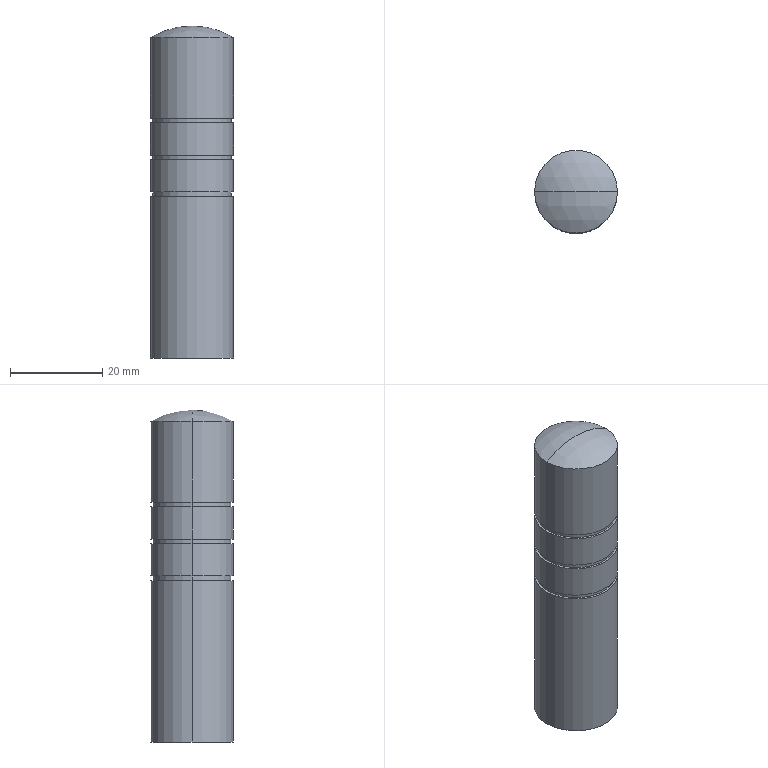Part | SolidWorks | features ICE 4, Extrusion 1, HoleWzd 1, Revolution 1 | 1 solid | 32 faces | box 18 x 18 x 71.992 mm | volume 12874 mm3 | cylinder 18 | plane 8 | cone 4 | sphere 2 | commonest cylinder face diameters 18 x8 17 x6 4.2 x2 14 x2
STEP:
#1=CARTESIAN_POINT('',(2.1,0.,32.425));
#2=VERTEX_POINT('',#1);
#3=CARTESIAN_POINT('',(-2.1,0.,32.425));
#4=VERTEX_POINT('',#3);
#5=CARTESIAN_POINT('',(0.,0.,32.425));
#6=DIRECTION('',(0.,0.,-1.));
#7=DIRECTION('',(-1.,0.,0.));
#8=AXIS2_PLACEMENT_3D('',#5,#6,#7);
#9=CIRCLE('',#8,2.1);
#10=EDGE_CURVE('',#2,#4,#9,.T.);
#11=ORIENTED_EDGE('',*,*,#10,.F.);
#12=CARTESIAN_POINT('',(2.525,0.,32.));
#13=VERTEX_POINT('',#12);
#14=CARTESIAN_POINT('',(2.525,0.,32.));
#15=DIRECTION('',(0.7071,0.,-0.7071));
#16=VECTOR('',#15,1000.);
#17=LINE('',#14,#16);
#18=EDGE_CURVE('',#2,#13,#17,.T.);
#19=ORIENTED_EDGE('',*,*,#18,.T.);
#20=CARTESIAN_POINT('',(-2.525,0.,32.));
#21=VERTEX_POINT('',#20);
#22=CARTESIAN_POINT('',(0.,0.,32.));
#23=DIRECTION('',(0.,0.,-1.));
#24=DIRECTION('',(-1.,0.,0.));
#25=AXIS2_PLACEMENT_3D('',#22,#23,#24);
#26=CIRCLE('',#25,2.525);
#27=EDGE_CURVE('',#13,#21,#26,.T.);
#28=ORIENTED_EDGE('',*,*,#27,.T.);
#29=CARTESIAN_POINT('',(-2.525,0.,32.));
#30=DIRECTION('',(-0.7071,0.,-0.7071));
#31=VECTOR('',#30,1000.);
#32=LINE('',#29,#31);
#33=EDGE_CURVE('',#4,#21,#32,.T.);
#34=ORIENTED_EDGE('',*,*,#33,.F.);
#35=EDGE_LOOP('',(#11,#19,#28,#34));
#36=FACE_OUTER_BOUND('',#35,.T.);
#37=CARTESIAN_POINT('',(0.,0.,32.));
#38=DIRECTION('',(0.,0.,-1.));
#39=DIRECTION('',(-1.,0.,0.));
#40=AXIS2_PLACEMENT_3D('',#37,#38,#39);
#41=CONICAL_SURFACE('',#40,2.525,0.7854);
#42=ADVANCED_FACE('',(#36),#41,.F.);
#43=CARTESIAN_POINT('',(2.1,0.,40.738));
#44=VERTEX_POINT('',#43);
#45=CARTESIAN_POINT('',(-2.1,0.,40.738));
#46=VERTEX_POINT('',#45);
#47=CARTESIAN_POINT('',(0.,0.,40.738));
#48=DIRECTION('',(0.,0.,-1.));
#49=DIRECTION('',(-1.,0.,0.));
#50=AXIS2_PLACEMENT_3D('',#47,#48,#49);
#51=CIRCLE('',#50,2.1);
#52=EDGE_CURVE('',#44,#46,#51,.T.);
#53=ORIENTED_EDGE('',*,*,#52,.F.);
#54=CARTESIAN_POINT('',(2.1,0.,32.));
#55=DIRECTION('',(0.,0.,-1.));
#56=VECTOR('',#55,1000.);
#57=LINE('',#54,#56);
#58=EDGE_CURVE('',#44,#2,#57,.T.);
#59=ORIENTED_EDGE('',*,*,#58,.T.);
#60=ORIENTED_EDGE('',*,*,#10,.T.);
#61=CARTESIAN_POINT('',(-2.1,0.,32.));
#62=DIRECTION('',(0.,0.,-1.));
#63=VECTOR('',#62,1000.);
#64=LINE('',#61,#63);
#65=EDGE_CURVE('',#46,#4,#64,.T.);
#66=ORIENTED_EDGE('',*,*,#65,.F.);
#67=EDGE_LOOP('',(#53,#59,#60,#66));
#68=FACE_OUTER_BOUND('',#67,.T.);
#69=CARTESIAN_POINT('',(0.,0.,32.));
#70=DIRECTION('',(0.,0.,-1.));
#71=DIRECTION('',(-1.,0.,0.));
#72=AXIS2_PLACEMENT_3D('',#69,#70,#71);
#73=CYLINDRICAL_SURFACE('',#72,2.1);
#74=ADVANCED_FACE('',(#68),#73,.F.);
#75=CARTESIAN_POINT('',(0.,0.,42.));
#76=VERTEX_POINT('',#75);
#77=CARTESIAN_POINT('',(-2.1,0.,40.738));
#78=DIRECTION('',(-0.8572,0.,-0.515));
#79=VECTOR('',#78,1000.);
#80=LINE('',#77,#79);
#81=EDGE_CURVE('',#76,#46,#80,.T.);
#82=ORIENTED_EDGE('',*,*,#81,.F.);
#83=CARTESIAN_POINT('',(2.1,0.,40.738));
#84=DIRECTION('',(0.8572,0.,-0.515));
#85=VECTOR('',#84,1000.);
#86=LINE('',#83,#85);
#87=EDGE_CURVE('',#76,#44,#86,.T.);
#88=ORIENTED_EDGE('',*,*,#87,.T.);
#89=ORIENTED_EDGE('',*,*,#52,.T.);
#90=EDGE_LOOP('',(#82,#88,#89));
#91=FACE_OUTER_BOUND('',#90,.T.);
#92=CARTESIAN_POINT('',(0.,0.,40.738));
#93=DIRECTION('',(0.,0.,-1.));
#94=DIRECTION('',(-1.,0.,0.));
#95=AXIS2_PLACEMENT_3D('',#92,#93,#94);
#96=CONICAL_SURFACE('',#95,2.1,1.03);
#97=ADVANCED_FACE('',(#91),#96,.F.);
#98=CARTESIAN_POINT('',(0.,0.,71.992));
#99=VERTEX_POINT('',#98);
#100=CARTESIAN_POINT('',(-9.,0.,69.5));
#101=VERTEX_POINT('',#100);
#102=CARTESIAN_POINT('',(0.,0.,54.492));
#103=DIRECTION('',(0.,-1.,0.));
#104=DIRECTION('',(0.,0.,-1.));
#105=AXIS2_PLACEMENT_3D('',#102,#103,#104);
#106=CIRCLE('',#105,17.5);
#107=EDGE_CURVE('',#99,#101,#106,.T.);
#108=ORIENTED_EDGE('',*,*,#107,.F.);
#109=CARTESIAN_POINT('',(9.,0.,69.5));
#110=VERTEX_POINT('',#109);
#111=CARTESIAN_POINT('',(0.,0.,54.492));
#112=DIRECTION('',(0.,1.,0.));
#113=DIRECTION('',(-1.,0.,0.));
#114=AXIS2_PLACEMENT_3D('',#111,#112,#113);
#115=CIRCLE('',#114,17.5);
#116=EDGE_CURVE('',#99,#110,#115,.T.);
#117=ORIENTED_EDGE('',*,*,#116,.T.);
#118=CARTESIAN_POINT('',(0.,0.,69.5));
#119=DIRECTION('',(0.,0.,1.));
#120=DIRECTION('',(1.,0.,0.));
#121=AXIS2_PLACEMENT_3D('',#118,#119,#120);
#122=CIRCLE('',#121,9.);
#123=EDGE_CURVE('',#110,#101,#122,.T.);
#124=ORIENTED_EDGE('',*,*,#123,.T.);
#125=EDGE_LOOP('',(#108,#117,#124));
#126=FACE_OUTER_BOUND('',#125,.T.);
#127=CARTESIAN_POINT('',(0.,0.,54.492));
#128=DIRECTION('',(0.,1.,0.));
#129=DIRECTION('',(-1.,0.,0.));
#130=AXIS2_PLACEMENT_3D('',#127,#128,#129);
#131=SPHERICAL_SURFACE('',#130,17.5);
#132=ADVANCED_FACE('',(#126),#131,.T.);
#133=ORIENTED_EDGE('',*,*,#123,.F.);
#134=CARTESIAN_POINT('',(9.,0.,52.));
#135=VERTEX_POINT('',#134);
#136=CARTESIAN_POINT('',(9.,0.,69.5));
#137=DIRECTION('',(0.,0.,-1.));
#138=VECTOR('',#137,1000.);
#139=LINE('',#136,#138);
#140=EDGE_CURVE('',#110,#135,#139,.T.);
#141=ORIENTED_EDGE('',*,*,#140,.T.);
#142=CARTESIAN_POINT('',(-9.,0.,52.));
#143=VERTEX_POINT('',#142);
#144=CARTESIAN_POINT('',(0.,0.,52.));
#145=DIRECTION('',(0.,0.,-1.));
#146=DIRECTION('',(-1.,0.,0.));
#147=AXIS2_PLACEMENT_3D('',#144,#145,#146);
#148=CIRCLE('',#147,9.);
#149=EDGE_CURVE('',#143,#135,#148,.T.);
#150=ORIENTED_EDGE('',*,*,#149,.F.);
#151=CARTESIAN_POINT('',(-9.,0.,69.5));
#152=DIRECTION('',(0.,0.,-1.));
#153=VECTOR('',#152,1000.);
#154=LINE('',#151,#153);
#155=EDGE_CURVE('',#101,#143,#154,.T.);
#156=ORIENTED_EDGE('',*,*,#155,.F.);
#157=EDGE_LOOP('',(#133,#141,#150,#156));
#158=FACE_OUTER_BOUND('',#157,.T.);
#159=CARTESIAN_POINT('',(0.,0.,69.5));
#160=DIRECTION('',(0.,0.,-1.));
#161=DIRECTION('',(-1.,0.,0.));
#162=AXIS2_PLACEMENT_3D('',#159,#160,#161);
#163=CYLINDRICAL_SURFACE('',#162,9.);
#164=ADVANCED_FACE('',(#158),#163,.T.);
#165=CARTESIAN_POINT('',(-8.5,0.,52.));
#166=VERTEX_POINT('',#165);
#167=CARTESIAN_POINT('',(8.5,0.,52.));
#168=VERTEX_POINT('',#167);
#169=CARTESIAN_POINT('',(0.,0.,52.));
#170=DIRECTION('',(0.,0.,-1.));
#171=DIRECTION('',(-1.,0.,0.));
#172=AXIS2_PLACEMENT_3D('',#169,#170,#171);
#173=CIRCLE('',#172,8.5);
#174=EDGE_CURVE('',#166,#168,#173,.T.);
#175=ORIENTED_EDGE('',*,*,#174,.T.);
#176=CARTESIAN_POINT('',(8.5,0.,51.));
#177=VERTEX_POINT('',#176);
#178=CARTESIAN_POINT('',(8.5,0.,52.));
#179=DIRECTION('',(0.,0.,-1.));
#180=VECTOR('',#179,1000.);
#181=LINE('',#178,#180);
#182=EDGE_CURVE('',#168,#177,#181,.T.);
#183=ORIENTED_EDGE('',*,*,#182,.T.);
#184=CARTESIAN_POINT('',(-8.5,0.,51.));
#185=VERTEX_POINT('',#184);
#186=CARTESIAN_POINT('',(0.,0.,51.));
#187=DIRECTION('',(0.,0.,-1.));
#188=DIRECTION('',(-1.,0.,0.));
#189=AXIS2_PLACEMENT_3D('',#186,#187,#188);
#190=CIRCLE('',#189,8.5);
#191=EDGE_CURVE('',#185,#177,#190,.T.);
#192=ORIENTED_EDGE('',*,*,#191,.F.);
#193=CARTESIAN_POINT('',(-8.5,0.,52.));
#194=DIRECTION('',(0.,0.,-1.));
#195=VECTOR('',#194,1000.);
#196=LINE('',#193,#195);
#197=EDGE_CURVE('',#166,#185,#196,.T.);
#198=ORIENTED_EDGE('',*,*,#197,.F.);
#199=EDGE_LOOP('',(#175,#183,#192,#198));
#200=FACE_OUTER_BOUND('',#199,.T.);
#201=CARTESIAN_POINT('',(0.,0.,52.));
#202=DIRECTION('',(0.,0.,-1.));
#203=DIRECTION('',(-1.,0.,0.));
#204=AXIS2_PLACEMENT_3D('',#201,#202,#203);
#205=CYLINDRICAL_SURFACE('',#204,8.5);
#206=ADVANCED_FACE('',(#200),#205,.T.);
#207=CARTESIAN_POINT('',(-9.,0.,51.));
#208=VERTEX_POINT('',#207);
#209=CARTESIAN_POINT('',(9.,0.,51.));
#210=VERTEX_POINT('',#209);
#211=CARTESIAN_POINT('',(0.,0.,51.));
#212=DIRECTION('',(0.,0.,-1.));
#213=DIRECTION('',(-1.,0.,0.));
#214=AXIS2_PLACEMENT_3D('',#211,#212,#213);
#215=CIRCLE('',#214,9.);
#216=EDGE_CURVE('',#208,#210,#215,.T.);
#217=ORIENTED_EDGE('',*,*,#216,.T.);
#218=CARTESIAN_POINT('',(9.,0.,44.));
#219=VERTEX_POINT('',#218);
#220=CARTESIAN_POINT('',(9.,0.,69.5));
#221=DIRECTION('',(0.,0.,-1.));
#222=VECTOR('',#221,1000.);
#223=LINE('',#220,#222);
#224=EDGE_CURVE('',#210,#219,#223,.T.);
#225=ORIENTED_EDGE('',*,*,#224,.T.);
#226=CARTESIAN_POINT('',(-9.,0.,44.));
#227=VERTEX_POINT('',#226);
#228=CARTESIAN_POINT('',(0.,0.,44.));
#229=DIRECTION('',(0.,0.,-1.));
#230=DIRECTION('',(-1.,0.,0.));
#231=AXIS2_PLACEMENT_3D('',#228,#229,#230);
#232=CIRCLE('',#231,9.);
#233=EDGE_CURVE('',#227,#219,#232,.T.);
#234=ORIENTED_EDGE('',*,*,#233,.F.);
#235=CARTESIAN_POINT('',(-9.,0.,69.5));
#236=DIRECTION('',(0.,0.,-1.));
#237=VECTOR('',#236,1000.);
#238=LINE('',#235,#237);
#239=EDGE_CURVE('',#208,#227,#238,.T.);
#240=ORIENTED_EDGE('',*,*,#239,.F.);
#241=EDGE_LOOP('',(#217,#225,#234,#240));
#242=FACE_OUTER_BOUND('',#241,.T.);
#243=CARTESIAN_POINT('',(0.,0.,69.5));
#244=DIRECTION('',(0.,0.,-1.));
#245=DIRECTION('',(-1.,0.,0.));
#246=AXIS2_PLACEMENT_3D('',#243,#244,#245);
#247=CYLINDRICAL_SURFACE('',#246,9.);
#248=ADVANCED_FACE('',(#242),#247,.T.);
#249=CARTESIAN_POINT('',(-8.5,0.,44.));
#250=VERTEX_POINT('',#249);
#251=CARTESIAN_POINT('',(8.5,0.,44.));
#252=VERTEX_POINT('',#251);
#253=CARTESIAN_POINT('',(0.,0.,44.));
#254=DIRECTION('',(0.,0.,-1.));
#255=DIRECTION('',(-1.,0.,0.));
#256=AXIS2_PLACEMENT_3D('',#253,#254,#255);
#257=CIRCLE('',#256,8.5);
#258=EDGE_CURVE('',#250,#252,#257,.T.);
#259=ORIENTED_EDGE('',*,*,#258,.T.);
#260=CARTESIAN_POINT('',(8.5,0.,43.));
#261=VERTEX_POINT('',#260);
#262=CARTESIAN_POINT('',(8.5,0.,44.));
#263=DIRECTION('',(0.,0.,-1.));
#264=VECTOR('',#263,1000.);
#265=LINE('',#262,#264);
#266=EDGE_CURVE('',#252,#261,#265,.T.);
#267=ORIENTED_EDGE('',*,*,#266,.T.);
#268=CARTESIAN_POINT('',(-8.5,0.,43.));
#269=VERTEX_POINT('',#268);
#270=CARTESIAN_POINT('',(0.,0.,43.));
#271=DIRECTION('',(0.,0.,-1.));
#272=DIRECTION('',(-1.,0.,0.));
#273=AXIS2_PLACEMENT_3D('',#270,#271,#272);
#274=CIRCLE('',#273,8.5);
#275=EDGE_CURVE('',#269,#261,#274,.T.);
#276=ORIENTED_EDGE('',*,*,#275,.F.);
#277=CARTESIAN_POINT('',(-8.5,0.,44.));
#278=DIRECTION('',(0.,0.,-1.));
#279=VECTOR('',#278,1000.);
#280=LINE('',#277,#279);
#281=EDGE_CURVE('',#250,#269,#280,.T.);
#282=ORIENTED_EDGE('',*,*,#281,.F.);
#283=EDGE_LOOP('',(#259,#267,#276,#282));
#284=FACE_OUTER_BOUND('',#283,.T.);
#285=CARTESIAN_POINT('',(0.,0.,44.));
#286=DIRECTION('',(0.,0.,-1.));
#287=DIRECTION('',(-1.,0.,0.));
#288=AXIS2_PLACEMENT_3D('',#285,#286,#287);
#289=CYLINDRICAL_SURFACE('',#288,8.5);
#290=ADVANCED_FACE('',(#284),#289,.T.);
#291=CARTESIAN_POINT('',(-9.,0.,43.));
#292=VERTEX_POINT('',#291);
#293=CARTESIAN_POINT('',(9.,0.,43.));
#294=VERTEX_POINT('',#293);
#295=CARTESIAN_POINT('',(0.,0.,43.));
#296=DIRECTION('',(0.,0.,-1.));
#297=DIRECTION('',(-1.,0.,0.));
#298=AXIS2_PLACEMENT_3D('',#295,#296,#297);
#299=CIRCLE('',#298,9.);
#300=EDGE_CURVE('',#292,#294,#299,.T.);
#301=ORIENTED_EDGE('',*,*,#300,.T.);
#302=CARTESIAN_POINT('',(9.,0.,36.));
#303=VERTEX_POINT('',#302);
#304=CARTESIAN_POINT('',(9.,0.,69.5));
#305=DIRECTION('',(0.,0.,-1.));
#306=VECTOR('',#305,1000.);
#307=LINE('',#304,#306);
#308=EDGE_CURVE('',#294,#303,#307,.T.);
#309=ORIENTED_EDGE('',*,*,#308,.T.);
#310=CARTESIAN_POINT('',(-9.,0.,36.));
#311=VERTEX_POINT('',#310);
#312=CARTESIAN_POINT('',(0.,0.,36.));
#313=DIRECTION('',(0.,0.,-1.));
#314=DIRECTION('',(-1.,0.,0.));
#315=AXIS2_PLACEMENT_3D('',#312,#313,#314);
#316=CIRCLE('',#315,9.);
#317=EDGE_CURVE('',#311,#303,#316,.T.);
#318=ORIENTED_EDGE('',*,*,#317,.F.);
#319=CARTESIAN_POINT('',(-9.,0.,69.5));
#320=DIRECTION('',(0.,0.,-1.));
#321=VECTOR('',#320,1000.);
#322=LINE('',#319,#321);
#323=EDGE_CURVE('',#292,#311,#322,.T.);
#324=ORIENTED_EDGE('',*,*,#323,.F.);
#325=EDGE_LOOP('',(#301,#309,#318,#324));
#326=FACE_OUTER_BOUND('',#325,.T.);
#327=CARTESIAN_POINT('',(0.,0.,69.5));
#328=DIRECTION('',(0.,0.,-1.));
#329=DIRECTION('',(-1.,0.,0.));
#330=AXIS2_PLACEMENT_3D('',#327,#328,#329);
#331=CYLINDRICAL_SURFACE('',#330,9.);
#332=ADVANCED_FACE('',(#326),#331,.T.);
#333=CARTESIAN_POINT('',(-8.5,0.,36.));
#334=VERTEX_POINT('',#333);
#335=CARTESIAN_POINT('',(8.5,0.,36.));
#336=VERTEX_POINT('',#335);
#337=CARTESIAN_POINT('',(0.,0.,36.));
#338=DIRECTION('',(0.,0.,-1.));
#339=DIRECTION('',(-1.,0.,0.));
#340=AXIS2_PLACEMENT_3D('',#337,#338,#339);
#341=CIRCLE('',#340,8.5);
#342=EDGE_CURVE('',#334,#336,#341,.T.);
#343=ORIENTED_EDGE('',*,*,#342,.T.);
#344=CARTESIAN_POINT('',(8.5,0.,35.));
#345=VERTEX_POINT('',#344);
#346=CARTESIAN_POINT('',(8.5,0.,36.));
#347=DIRECTION('',(0.,0.,-1.));
#348=VECTOR('',#347,1000.);
#349=LINE('',#346,#348);
#350=EDGE_CURVE('',#336,#345,#349,.T.);
#351=ORIENTED_EDGE('',*,*,#350,.T.);
#352=CARTESIAN_POINT('',(-8.5,0.,35.));
#353=VERTEX_POINT('',#352);
#354=CARTESIAN_POINT('',(0.,0.,35.));
#355=DIRECTION('',(0.,0.,-1.));
#356=DIRECTION('',(-1.,0.,0.));
#357=AXIS2_PLACEMENT_3D('',#354,#355,#356);
#358=CIRCLE('',#357,8.5);
#359=EDGE_CURVE('',#353,#345,#358,.T.);
#360=ORIENTED_EDGE('',*,*,#359,.F.);
#361=CARTESIAN_POINT('',(-8.5,0.,36.));
#362=DIRECTION('',(0.,0.,-1.));
#363=VECTOR('',#362,1000.);
#364=LINE('',#361,#363);
#365=EDGE_CURVE('',#334,#353,#364,.T.);
#366=ORIENTED_EDGE('',*,*,#365,.F.);
#367=EDGE_LOOP('',(#343,#351,#360,#366));
#368=FACE_OUTER_BOUND('',#367,.T.);
#369=CARTESIAN_POINT('',(0.,0.,36.));
#370=DIRECTION('',(0.,0.,-1.));
#371=DIRECTION('',(-1.,0.,0.));
#372=AXIS2_PLACEMENT_3D('',#369,#370,#371);
#373=CYLINDRICAL_SURFACE('',#372,8.5);
#374=ADVANCED_FACE('',(#368),#373,.T.);
#375=CARTESIAN_POINT('',(7.,0.,32.));
#376=VERTEX_POINT('',#375);
#377=CARTESIAN_POINT('',(-7.,0.,32.));
#378=VERTEX_POINT('',#377);
#379=CARTESIAN_POINT('',(0.,0.,32.));
#380=DIRECTION('',(0.,0.,-1.));
#381=DIRECTION('',(-1.,0.,0.));
#382=AXIS2_PLACEMENT_3D('',#379,#380,#381);
#383=CIRCLE('',#382,7.);
#384=EDGE_CURVE('',#376,#378,#383,.T.);
#385=ORIENTED_EDGE('',*,*,#384,.F.);
#386=CARTESIAN_POINT('',(7.,0.,0.));
#387=VERTEX_POINT('',#386);
#388=CARTESIAN_POINT('',(7.,0.,32.));
#389=DIRECTION('',(0.,0.,-1.));
#390=VECTOR('',#389,1000.);
#391=LINE('',#388,#390);
#392=EDGE_CURVE('',#376,#387,#391,.T.);
#393=ORIENTED_EDGE('',*,*,#392,.T.);
#394=CARTESIAN_POINT('',(-7.,0.,0.));
#395=VERTEX_POINT('',#394);
#396=CARTESIAN_POINT('',(0.,0.,0.));
#397=DIRECTION('',(0.,0.,-1.));
#398=DIRECTION('',(-1.,0.,0.));
#399=AXIS2_PLACEMENT_3D('',#396,#397,#398);
#400=CIRCLE('',#399,7.);
#401=EDGE_CURVE('',#387,#395,#400,.T.);
#402=ORIENTED_EDGE('',*,*,#401,.T.);
#403=CARTESIAN_POINT('',(-7.,0.,32.));
#404=DIRECTION('',(0.,0.,-1.));
#405=VECTOR('',#404,1000.);
#406=LINE('',#403,#405);
#407=EDGE_CURVE('',#378,#395,#406,.T.);
#408=ORIENTED_EDGE('',*,*,#407,.F.);
#409=EDGE_LOOP('',(#385,#393,#402,#408));
#410=FACE_OUTER_BOUND('',#409,.T.);
#411=CARTESIAN_POINT('',(0.,0.,32.));
#412=DIRECTION('',(0.,0.,-1.));
#413=DIRECTION('',(-1.,0.,0.));
#414=AXIS2_PLACEMENT_3D('',#411,#412,#413);
#415=CYLINDRICAL_SURFACE('',#414,7.);
#416=ADVANCED_FACE('',(#410),#415,.F.);
#417=CARTESIAN_POINT('',(-9.,0.,35.));
#418=VERTEX_POINT('',#417);
#419=CARTESIAN_POINT('',(9.,0.,35.));
#420=VERTEX_POINT('',#419);
#421=CARTESIAN_POINT('',(0.,0.,35.));
#422=DIRECTION('',(0.,0.,-1.));
#423=DIRECTION('',(-1.,0.,0.));
#424=AXIS2_PLACEMENT_3D('',#421,#422,#423);
#425=CIRCLE('',#424,9.);
#426=EDGE_CURVE('',#418,#420,#425,.T.);
#427=ORIENTED_EDGE('',*,*,#426,.T.);
#428=CARTESIAN_POINT('',(9.,0.,0.));
#429=VERTEX_POINT('',#428);
#430=CARTESIAN_POINT('',(9.,0.,69.5));
#431=DIRECTION('',(0.,0.,-1.));
#432=VECTOR('',#431,1000.);
#433=LINE('',#430,#432);
#434=EDGE_CURVE('',#420,#429,#433,.T.);
#435=ORIENTED_EDGE('',*,*,#434,.T.);
#436=CARTESIAN_POINT('',(-9.,0.,0.));
#437=VERTEX_POINT('',#436);
#438=CARTESIAN_POINT('',(0.,0.,0.));
#439=DIRECTION('',(0.,0.,1.));
#440=DIRECTION('',(1.,0.,0.));
#441=AXIS2_PLACEMENT_3D('',#438,#439,#440);
#442=CIRCLE('',#441,9.);
#443=EDGE_CURVE('',#429,#437,#442,.T.);
#444=ORIENTED_EDGE('',*,*,#443,.T.);
#445=CARTESIAN_POINT('',(-9.,0.,69.5));
#446=DIRECTION('',(0.,0.,-1.));
#447=VECTOR('',#446,1000.);
#448=LINE('',#445,#447);
#449=EDGE_CURVE('',#418,#437,#448,.T.);
#450=ORIENTED_EDGE('',*,*,#449,.F.);
#451=EDGE_LOOP('',(#427,#435,#444,#450));
#452=FACE_OUTER_BOUND('',#451,.T.);
#453=CARTESIAN_POINT('',(0.,0.,69.5));
#454=DIRECTION('',(0.,0.,-1.));
#455=DIRECTION('',(-1.,0.,0.));
#456=AXIS2_PLACEMENT_3D('',#453,#454,#455);
#457=CYLINDRICAL_SURFACE('',#456,9.);
#458=ADVANCED_FACE('',(#452),#457,.T.);
#459=ORIENTED_EDGE('',*,*,#434,.F.);
#460=CARTESIAN_POINT('',(0.,0.,35.));
#461=DIRECTION('',(0.,0.,-1.));
#462=DIRECTION('',(-1.,0.,0.));
#463=AXIS2_PLACEMENT_3D('',#460,#461,#462);
#464=CIRCLE('',#463,9.);
#465=EDGE_CURVE('',#420,#418,#464,.T.);
#466=ORIENTED_EDGE('',*,*,#465,.T.);
#467=ORIENTED_EDGE('',*,*,#449,.T.);
#468=CARTESIAN_POINT('',(0.,0.,0.));
#469=DIRECTION('',(0.,0.,1.));
#470=DIRECTION('',(1.,0.,0.));
#471=AXIS2_PLACEMENT_3D('',#468,#469,#470);
#472=CIRCLE('',#471,9.);
#473=EDGE_CURVE('',#437,#429,#472,.T.);
#474=ORIENTED_EDGE('',*,*,#473,.T.);
#475=EDGE_LOOP('',(#459,#466,#467,#474));
#476=FACE_OUTER_BOUND('',#475,.T.);
#477=CARTESIAN_POINT('',(0.,0.,69.5));
#478=DIRECTION('',(0.,0.,-1.));
#479=DIRECTION('',(-1.,0.,0.));
#480=AXIS2_PLACEMENT_3D('',#477,#478,#479);
#481=CYLINDRICAL_SURFACE('',#480,9.);
#482=ADVANCED_FACE('',(#476),#481,.T.);
#483=CARTESIAN_POINT('',(0.,0.,0.));
#484=DIRECTION('',(0.,0.,-1.));
#485=DIRECTION('',(-1.,0.,0.));
#486=AXIS2_PLACEMENT_3D('',#483,#484,#485);
#487=CIRCLE('',#486,7.);
#488=EDGE_CURVE('',#395,#387,#487,.T.);
#489=ORIENTED_EDGE('',*,*,#488,.F.);
#490=ORIENTED_EDGE('',*,*,#401,.F.);
#491=EDGE_LOOP('',(#489,#490));
#492=FACE_BOUND('',#491,.T.);
#493=ORIENTED_EDGE('',*,*,#473,.F.);
#494=ORIENTED_EDGE('',*,*,#443,.F.);
#495=EDGE_LOOP('',(#493,#494));
#496=FACE_OUTER_BOUND('',#495,.T.);
#497=CARTESIAN_POINT('',(0.,0.,0.));
#498=DIRECTION('',(0.,0.,1.));
#499=DIRECTION('',(1.,0.,0.));
#500=AXIS2_PLACEMENT_3D('',#497,#498,#499);
#501=PLANE('',#500);
#502=ADVANCED_FACE('',(#492,#496),#501,.F.);
#503=ORIENTED_EDGE('',*,*,#392,.F.);
#504=CARTESIAN_POINT('',(0.,0.,32.));
#505=DIRECTION('',(0.,0.,-1.));
#506=DIRECTION('',(-1.,0.,0.));
#507=AXIS2_PLACEMENT_3D('',#504,#505,#506);
#508=CIRCLE('',#507,7.);
#509=EDGE_CURVE('',#378,#376,#508,.T.);
#510=ORIENTED_EDGE('',*,*,#509,.F.);
#511=ORIENTED_EDGE('',*,*,#407,.T.);
#512=ORIENTED_EDGE('',*,*,#488,.T.);
#513=EDGE_LOOP('',(#503,#510,#511,#512));
#514=FACE_OUTER_BOUND('',#513,.T.);
#515=CARTESIAN_POINT('',(0.,0.,32.));
#516=DIRECTION('',(0.,0.,-1.));
#517=DIRECTION('',(-1.,0.,0.));
#518=AXIS2_PLACEMENT_3D('',#515,#516,#517);
#519=CYLINDRICAL_SURFACE('',#518,7.);
#520=ADVANCED_FACE('',(#514),#519,.F.);
#521=CARTESIAN_POINT('',(0.,0.,32.));
#522=DIRECTION('',(0.,0.,-1.));
#523=DIRECTION('',(-1.,0.,0.));
#524=AXIS2_PLACEMENT_3D('',#521,#522,#523);
#525=CIRCLE('',#524,2.525);
#526=EDGE_CURVE('',#21,#13,#525,.T.);
#527=ORIENTED_EDGE('',*,*,#526,.F.);
#528=ORIENTED_EDGE('',*,*,#27,.F.);
#529=EDGE_LOOP('',(#527,#528));
#530=FACE_BOUND('',#529,.T.);
#531=ORIENTED_EDGE('',*,*,#509,.T.);
#532=ORIENTED_EDGE('',*,*,#384,.T.);
#533=EDGE_LOOP('',(#531,#532));
#534=FACE_OUTER_BOUND('',#533,.T.);
#535=CARTESIAN_POINT('',(0.,0.,32.));
#536=DIRECTION('',(0.,0.,-1.));
#537=DIRECTION('',(-1.,0.,0.));
#538=AXIS2_PLACEMENT_3D('',#535,#536,#537);
#539=PLANE('',#538);
#540=ADVANCED_FACE('',(#530,#534),#539,.T.);
#541=ORIENTED_EDGE('',*,*,#342,.F.);
#542=CARTESIAN_POINT('',(0.,0.,36.));
#543=DIRECTION('',(0.,0.,-1.));
#544=DIRECTION('',(-1.,0.,0.));
#545=AXIS2_PLACEMENT_3D('',#542,#543,#544);
#546=CIRCLE('',#545,8.5);
#547=EDGE_CURVE('',#336,#334,#546,.T.);
#548=ORIENTED_EDGE('',*,*,#547,.F.);
#549=EDGE_LOOP('',(#541,#548));
#550=FACE_BOUND('',#549,.T.);
#551=ORIENTED_EDGE('',*,*,#317,.T.);
#552=CARTESIAN_POINT('',(0.,0.,36.));
#553=DIRECTION('',(0.,0.,-1.));
#554=DIRECTION('',(-1.,0.,0.));
#555=AXIS2_PLACEMENT_3D('',#552,#553,#554);
#556=CIRCLE('',#555,9.);
#557=EDGE_CURVE('',#303,#311,#556,.T.);
#558=ORIENTED_EDGE('',*,*,#557,.T.);
#559=EDGE_LOOP('',(#551,#558));
#560=FACE_OUTER_BOUND('',#559,.T.);
#561=CARTESIAN_POINT('',(0.,0.,36.));
#562=DIRECTION('',(0.,0.,-1.));
#563=DIRECTION('',(-1.,0.,0.));
#564=AXIS2_PLACEMENT_3D('',#561,#562,#563);
#565=PLANE('',#564);
#566=ADVANCED_FACE('',(#550,#560),#565,.T.);
#567=ORIENTED_EDGE('',*,*,#359,.T.);
#568=CARTESIAN_POINT('',(0.,0.,35.));
#569=DIRECTION('',(0.,0.,-1.));
#570=DIRECTION('',(-1.,0.,0.));
#571=AXIS2_PLACEMENT_3D('',#568,#569,#570);
#572=CIRCLE('',#571,8.5);
#573=EDGE_CURVE('',#345,#353,#572,.T.);
#574=ORIENTED_EDGE('',*,*,#573,.T.);
#575=EDGE_LOOP('',(#567,#574));
#576=FACE_BOUND('',#575,.T.);
#577=ORIENTED_EDGE('',*,*,#426,.F.);
#578=ORIENTED_EDGE('',*,*,#465,.F.);
#579=EDGE_LOOP('',(#577,#578));
#580=FACE_OUTER_BOUND('',#579,.T.);
#581=CARTESIAN_POINT('',(0.,0.,35.));
#582=DIRECTION('',(0.,0.,-1.));
#583=DIRECTION('',(-1.,0.,0.));
#584=AXIS2_PLACEMENT_3D('',#581,#582,#583);
#585=PLANE('',#584);
#586=ADVANCED_FACE('',(#576,#580),#585,.F.);
#587=ORIENTED_EDGE('',*,*,#350,.F.);
#588=ORIENTED_EDGE('',*,*,#547,.T.);
#589=ORIENTED_EDGE('',*,*,#365,.T.);
#590=ORIENTED_EDGE('',*,*,#573,.F.);
#591=EDGE_LOOP('',(#587,#588,#589,#590));
#592=FACE_OUTER_BOUND('',#591,.T.);
#593=CARTESIAN_POINT('',(0.,0.,36.));
#594=DIRECTION('',(0.,0.,-1.));
#595=DIRECTION('',(-1.,0.,0.));
#596=AXIS2_PLACEMENT_3D('',#593,#594,#595);
#597=CYLINDRICAL_SURFACE('',#596,8.5);
#598=ADVANCED_FACE('',(#592),#597,.T.);
#599=ORIENTED_EDGE('',*,*,#308,.F.);
#600=CARTESIAN_POINT('',(0.,0.,43.));
#601=DIRECTION('',(0.,0.,-1.));
#602=DIRECTION('',(-1.,0.,0.));
#603=AXIS2_PLACEMENT_3D('',#600,#601,#602);
#604=CIRCLE('',#603,9.);
#605=EDGE_CURVE('',#294,#292,#604,.T.);
#606=ORIENTED_EDGE('',*,*,#605,.T.);
#607=ORIENTED_EDGE('',*,*,#323,.T.);
#608=ORIENTED_EDGE('',*,*,#557,.F.);
#609=EDGE_LOOP('',(#599,#606,#607,#608));
#610=FACE_OUTER_BOUND('',#609,.T.);
#611=CARTESIAN_POINT('',(0.,0.,69.5));
#612=DIRECTION('',(0.,0.,-1.));
#613=DIRECTION('',(-1.,0.,0.));
#614=AXIS2_PLACEMENT_3D('',#611,#612,#613);
#615=CYLINDRICAL_SURFACE('',#614,9.);
#616=ADVANCED_FACE('',(#610),#615,.T.);
#617=ORIENTED_EDGE('',*,*,#258,.F.);
#618=CARTESIAN_POINT('',(0.,0.,44.));
#619=DIRECTION('',(0.,0.,-1.));
#620=DIRECTION('',(-1.,0.,0.));
#621=AXIS2_PLACEMENT_3D('',#618,#619,#620);
#622=CIRCLE('',#621,8.5);
#623=EDGE_CURVE('',#252,#250,#622,.T.);
#624=ORIENTED_EDGE('',*,*,#623,.F.);
#625=EDGE_LOOP('',(#617,#624));
#626=FACE_BOUND('',#625,.T.);
#627=ORIENTED_EDGE('',*,*,#233,.T.);
#628=CARTESIAN_POINT('',(0.,0.,44.));
#629=DIRECTION('',(0.,0.,-1.));
#630=DIRECTION('',(-1.,0.,0.));
#631=AXIS2_PLACEMENT_3D('',#628,#629,#630);
#632=CIRCLE('',#631,9.);
#633=EDGE_CURVE('',#219,#227,#632,.T.);
#634=ORIENTED_EDGE('',*,*,#633,.T.);
#635=EDGE_LOOP('',(#627,#634));
#636=FACE_OUTER_BOUND('',#635,.T.);
#637=CARTESIAN_POINT('',(0.,0.,44.));
#638=DIRECTION('',(0.,0.,-1.));
#639=DIRECTION('',(-1.,0.,0.));
#640=AXIS2_PLACEMENT_3D('',#637,#638,#639);
#641=PLANE('',#640);
#642=ADVANCED_FACE('',(#626,#636),#641,.T.);
#643=ORIENTED_EDGE('',*,*,#275,.T.);
#644=CARTESIAN_POINT('',(0.,0.,43.));
#645=DIRECTION('',(0.,0.,-1.));
#646=DIRECTION('',(-1.,0.,0.));
#647=AXIS2_PLACEMENT_3D('',#644,#645,#646);
#648=CIRCLE('',#647,8.5);
#649=EDGE_CURVE('',#261,#269,#648,.T.);
#650=ORIENTED_EDGE('',*,*,#649,.T.);
#651=EDGE_LOOP('',(#643,#650));
#652=FACE_BOUND('',#651,.T.);
#653=ORIENTED_EDGE('',*,*,#300,.F.);
#654=ORIENTED_EDGE('',*,*,#605,.F.);
#655=EDGE_LOOP('',(#653,#654));
#656=FACE_OUTER_BOUND('',#655,.T.);
#657=CARTESIAN_POINT('',(0.,0.,43.));
#658=DIRECTION('',(0.,0.,-1.));
#659=DIRECTION('',(-1.,0.,0.));
#660=AXIS2_PLACEMENT_3D('',#657,#658,#659);
#661=PLANE('',#660);
#662=ADVANCED_FACE('',(#652,#656),#661,.F.);
#663=ORIENTED_EDGE('',*,*,#266,.F.);
#664=ORIENTED_EDGE('',*,*,#623,.T.);
#665=ORIENTED_EDGE('',*,*,#281,.T.);
#666=ORIENTED_EDGE('',*,*,#649,.F.);
#667=EDGE_LOOP('',(#663,#664,#665,#666));
#668=FACE_OUTER_BOUND('',#667,.T.);
#669=CARTESIAN_POINT('',(0.,0.,44.));
#670=DIRECTION('',(0.,0.,-1.));
#671=DIRECTION('',(-1.,0.,0.));
#672=AXIS2_PLACEMENT_3D('',#669,#670,#671);
#673=CYLINDRICAL_SURFACE('',#672,8.5);
#674=ADVANCED_FACE('',(#668),#673,.T.);
#675=ORIENTED_EDGE('',*,*,#224,.F.);
#676=CARTESIAN_POINT('',(0.,0.,51.));
#677=DIRECTION('',(0.,0.,-1.));
#678=DIRECTION('',(-1.,0.,0.));
#679=AXIS2_PLACEMENT_3D('',#676,#677,#678);
#680=CIRCLE('',#679,9.);
#681=EDGE_CURVE('',#210,#208,#680,.T.);
#682=ORIENTED_EDGE('',*,*,#681,.T.);
#683=ORIENTED_EDGE('',*,*,#239,.T.);
#684=ORIENTED_EDGE('',*,*,#633,.F.);
#685=EDGE_LOOP('',(#675,#682,#683,#684));
#686=FACE_OUTER_BOUND('',#685,.T.);
#687=CARTESIAN_POINT('',(0.,0.,69.5));
#688=DIRECTION('',(0.,0.,-1.));
#689=DIRECTION('',(-1.,0.,0.));
#690=AXIS2_PLACEMENT_3D('',#687,#688,#689);
#691=CYLINDRICAL_SURFACE('',#690,9.);
#692=ADVANCED_FACE('',(#686),#691,.T.);
#693=ORIENTED_EDGE('',*,*,#174,.F.);
#694=CARTESIAN_POINT('',(0.,0.,52.));
#695=DIRECTION('',(0.,0.,-1.));
#696=DIRECTION('',(-1.,0.,0.));
#697=AXIS2_PLACEMENT_3D('',#694,#695,#696);
#698=CIRCLE('',#697,8.5);
#699=EDGE_CURVE('',#168,#166,#698,.T.);
#700=ORIENTED_EDGE('',*,*,#699,.F.);
#701=EDGE_LOOP('',(#693,#700));
#702=FACE_BOUND('',#701,.T.);
#703=ORIENTED_EDGE('',*,*,#149,.T.);
#704=CARTESIAN_POINT('',(0.,0.,52.));
#705=DIRECTION('',(0.,0.,-1.));
#706=DIRECTION('',(-1.,0.,0.));
#707=AXIS2_PLACEMENT_3D('',#704,#705,#706);
#708=CIRCLE('',#707,9.);
#709=EDGE_CURVE('',#135,#143,#708,.T.);
#710=ORIENTED_EDGE('',*,*,#709,.T.);
#711=EDGE_LOOP('',(#703,#710));
#712=FACE_OUTER_BOUND('',#711,.T.);
#713=CARTESIAN_POINT('',(0.,0.,52.));
#714=DIRECTION('',(0.,0.,-1.));
#715=DIRECTION('',(-1.,0.,0.));
#716=AXIS2_PLACEMENT_3D('',#713,#714,#715);
#717=PLANE('',#716);
#718=ADVANCED_FACE('',(#702,#712),#717,.T.);
#719=ORIENTED_EDGE('',*,*,#191,.T.);
#720=CARTESIAN_POINT('',(0.,0.,51.));
#721=DIRECTION('',(0.,0.,-1.));
#722=DIRECTION('',(-1.,0.,0.));
#723=AXIS2_PLACEMENT_3D('',#720,#721,#722);
#724=CIRCLE('',#723,8.5);
#725=EDGE_CURVE('',#177,#185,#724,.T.);
#726=ORIENTED_EDGE('',*,*,#725,.T.);
#727=EDGE_LOOP('',(#719,#726));
#728=FACE_BOUND('',#727,.T.);
#729=ORIENTED_EDGE('',*,*,#216,.F.);
#730=ORIENTED_EDGE('',*,*,#681,.F.);
#731=EDGE_LOOP('',(#729,#730));
#732=FACE_OUTER_BOUND('',#731,.T.);
#733=CARTESIAN_POINT('',(0.,0.,51.));
#734=DIRECTION('',(0.,0.,-1.));
#735=DIRECTION('',(-1.,0.,0.));
#736=AXIS2_PLACEMENT_3D('',#733,#734,#735);
#737=PLANE('',#736);
#738=ADVANCED_FACE('',(#728,#732),#737,.F.);
#739=ORIENTED_EDGE('',*,*,#182,.F.);
#740=ORIENTED_EDGE('',*,*,#699,.T.);
#741=ORIENTED_EDGE('',*,*,#197,.T.);
#742=ORIENTED_EDGE('',*,*,#725,.F.);
#743=EDGE_LOOP('',(#739,#740,#741,#742));
#744=FACE_OUTER_BOUND('',#743,.T.);
#745=CARTESIAN_POINT('',(0.,0.,52.));
#746=DIRECTION('',(0.,0.,-1.));
#747=DIRECTION('',(-1.,0.,0.));
#748=AXIS2_PLACEMENT_3D('',#745,#746,#747);
#749=CYLINDRICAL_SURFACE('',#748,8.5);
#750=ADVANCED_FACE('',(#744),#749,.T.);
#751=ORIENTED_EDGE('',*,*,#140,.F.);
#752=CARTESIAN_POINT('',(0.,0.,69.5));
#753=DIRECTION('',(0.,0.,1.));
#754=DIRECTION('',(1.,0.,0.));
#755=AXIS2_PLACEMENT_3D('',#752,#753,#754);
#756=CIRCLE('',#755,9.);
#757=EDGE_CURVE('',#101,#110,#756,.T.);
#758=ORIENTED_EDGE('',*,*,#757,.F.);
#759=ORIENTED_EDGE('',*,*,#155,.T.);
#760=ORIENTED_EDGE('',*,*,#709,.F.);
#761=EDGE_LOOP('',(#751,#758,#759,#760));
#762=FACE_OUTER_BOUND('',#761,.T.);
#763=CARTESIAN_POINT('',(0.,0.,69.5));
#764=DIRECTION('',(0.,0.,-1.));
#765=DIRECTION('',(-1.,0.,0.));
#766=AXIS2_PLACEMENT_3D('',#763,#764,#765);
#767=CYLINDRICAL_SURFACE('',#766,9.);
#768=ADVANCED_FACE('',(#762),#767,.T.);
#769=ORIENTED_EDGE('',*,*,#116,.F.);
#770=ORIENTED_EDGE('',*,*,#107,.T.);
#771=ORIENTED_EDGE('',*,*,#757,.T.);
#772=EDGE_LOOP('',(#769,#770,#771));
#773=FACE_OUTER_BOUND('',#772,.T.);
#774=CARTESIAN_POINT('',(0.,0.,54.492));
#775=DIRECTION('',(0.,1.,0.));
#776=DIRECTION('',(-1.,0.,0.));
#777=AXIS2_PLACEMENT_3D('',#774,#775,#776);
#778=SPHERICAL_SURFACE('',#777,17.5);
#779=ADVANCED_FACE('',(#773),#778,.T.);
#780=ORIENTED_EDGE('',*,*,#87,.F.);
#781=ORIENTED_EDGE('',*,*,#81,.T.);
#782=CARTESIAN_POINT('',(0.,0.,40.738));
#783=DIRECTION('',(0.,0.,-1.));
#784=DIRECTION('',(-1.,0.,0.));
#785=AXIS2_PLACEMENT_3D('',#782,#783,#784);
#786=CIRCLE('',#785,2.1);
#787=EDGE_CURVE('',#46,#44,#786,.T.);
#788=ORIENTED_EDGE('',*,*,#787,.T.);
#789=EDGE_LOOP('',(#780,#781,#788));
#790=FACE_OUTER_BOUND('',#789,.T.);
#791=CARTESIAN_POINT('',(0.,0.,40.738));
#792=DIRECTION('',(0.,0.,-1.));
#793=DIRECTION('',(-1.,0.,0.));
#794=AXIS2_PLACEMENT_3D('',#791,#792,#793);
#795=CONICAL_SURFACE('',#794,2.1,1.03);
#796=ADVANCED_FACE('',(#790),#795,.F.);
#797=ORIENTED_EDGE('',*,*,#58,.F.);
#798=ORIENTED_EDGE('',*,*,#787,.F.);
#799=ORIENTED_EDGE('',*,*,#65,.T.);
#800=CARTESIAN_POINT('',(0.,0.,32.425));
#801=DIRECTION('',(0.,0.,-1.));
#802=DIRECTION('',(-1.,0.,0.));
#803=AXIS2_PLACEMENT_3D('',#800,#801,#802);
#804=CIRCLE('',#803,2.1);
#805=EDGE_CURVE('',#4,#2,#804,.T.);
#806=ORIENTED_EDGE('',*,*,#805,.T.);
#807=EDGE_LOOP('',(#797,#798,#799,#806));
#808=FACE_OUTER_BOUND('',#807,.T.);
#809=CARTESIAN_POINT('',(0.,0.,32.));
#810=DIRECTION('',(0.,0.,-1.));
#811=DIRECTION('',(-1.,0.,0.));
#812=AXIS2_PLACEMENT_3D('',#809,#810,#811);
#813=CYLINDRICAL_SURFACE('',#812,2.1);
#814=ADVANCED_FACE('',(#808),#813,.F.);
#815=ORIENTED_EDGE('',*,*,#18,.F.);
#816=ORIENTED_EDGE('',*,*,#805,.F.);
#817=ORIENTED_EDGE('',*,*,#33,.T.);
#818=ORIENTED_EDGE('',*,*,#526,.T.);
#819=EDGE_LOOP('',(#815,#816,#817,#818));
#820=FACE_OUTER_BOUND('',#819,.T.);
#821=CARTESIAN_POINT('',(0.,0.,32.));
#822=DIRECTION('',(0.,0.,-1.));
#823=DIRECTION('',(-1.,0.,0.));
#824=AXIS2_PLACEMENT_3D('',#821,#822,#823);
#825=CONICAL_SURFACE('',#824,2.525,0.7854);
#826=ADVANCED_FACE('',(#820),#825,.F.);
#827=CLOSED_SHELL('',(#42,#74,#97,#132,#164,#206,#248,#290,#332,#374,#416,#458,#482,#502,#520,#540,#566,#586,#598,#616,#642,#662,#674,#692,#718,#738,#750,#768,#779,#796,#814,#826));
#828=MANIFOLD_SOLID_BREP('',#827);
#829=CARTESIAN_POINT('',(0.,0.,0.));
#830=DIRECTION('',(0.,0.,1.));
#831=DIRECTION('',(1.,0.,0.));
#832=AXIS2_PLACEMENT_3D('',#829,#830,#831);
#833=(LENGTH_UNIT()NAMED_UNIT(*)SI_UNIT(.MILLI.,.METRE.));
#834=UNCERTAINTY_MEASURE_WITH_UNIT(LENGTH_MEASURE(0.00001),#833,'','');
#835=(NAMED_UNIT(*)PLANE_ANGLE_UNIT()SI_UNIT($,.RADIAN.));
#836=(NAMED_UNIT(*)SI_UNIT($,.STERADIAN.)SOLID_ANGLE_UNIT());
#837=(GEOMETRIC_REPRESENTATION_CONTEXT(3)GLOBAL_UNCERTAINTY_ASSIGNED_CONTEXT((#834))GLOBAL_UNIT_ASSIGNED_CONTEXT((#833,#835,#836))REPRESENTATION_CONTEXT('',''));
#838=ADVANCED_BREP_SHAPE_REPRESENTATION('',(#828,#832),#837);